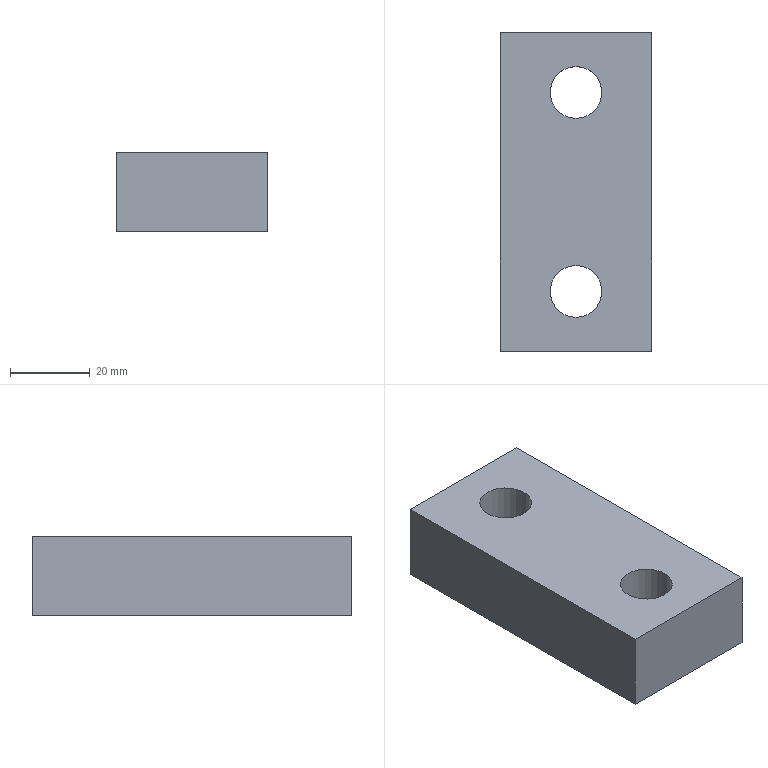Part | NX | features solid 2 | 1 solid | 12 faces | box 38 x 80 x 20 mm | volume 51862 mm3 | plane 8 | cylinder 4 | commonest cylinder face diameters 13 x2 20 x2
STEP:
#1=CARTESIAN_POINT('',(86.,140.,255.));
#2=VERTEX_POINT('',#1);
#3=CARTESIAN_POINT('',(76.,140.,255.));
#4=DIRECTION('',(0.,0.,-1.));
#5=DIRECTION('',(1.,0.,0.));
#6=AXIS2_PLACEMENT_3D('',#3,#4,#5);
#7=CIRCLE('',#6,10.);
#8=EDGE_CURVE('',#2,#2,#7,.F.);
#9=ORIENTED_EDGE('',*,*,#8,.T.);
#10=EDGE_LOOP('',(#9));
#11=FACE_BOUND('',#10,.T.);
#12=CARTESIAN_POINT('',(86.,190.,255.));
#13=VERTEX_POINT('',#12);
#14=CARTESIAN_POINT('',(76.,190.,255.));
#15=DIRECTION('',(0.,0.,-1.));
#16=DIRECTION('',(1.,0.,0.));
#17=AXIS2_PLACEMENT_3D('',#14,#15,#16);
#18=CIRCLE('',#17,10.);
#19=EDGE_CURVE('',#13,#13,#18,.F.);
#20=ORIENTED_EDGE('',*,*,#19,.T.);
#21=EDGE_LOOP('',(#20));
#22=FACE_BOUND('',#21,.T.);
#23=CARTESIAN_POINT('',(95.,125.,255.));
#24=VERTEX_POINT('',#23);
#25=CARTESIAN_POINT('',(95.,205.,255.));
#26=VERTEX_POINT('',#25);
#27=CARTESIAN_POINT('',(95.,165.,255.));
#28=DIRECTION('',(0.,1.,0.));
#29=VECTOR('',#28,1000.);
#30=LINE('',#27,#29);
#31=EDGE_CURVE('',#24,#26,#30,.T.);
#32=ORIENTED_EDGE('',*,*,#31,.F.);
#33=CARTESIAN_POINT('',(57.,125.,255.));
#34=VERTEX_POINT('',#33);
#35=CARTESIAN_POINT('',(75.,125.,255.));
#36=DIRECTION('',(1.,0.,0.));
#37=VECTOR('',#36,1000.);
#38=LINE('',#35,#37);
#39=EDGE_CURVE('',#34,#24,#38,.T.);
#40=ORIENTED_EDGE('',*,*,#39,.F.);
#41=CARTESIAN_POINT('',(57.,205.,255.));
#42=VERTEX_POINT('',#41);
#43=CARTESIAN_POINT('',(57.,165.,255.));
#44=DIRECTION('',(0.,-1.,0.));
#45=VECTOR('',#44,1000.);
#46=LINE('',#43,#45);
#47=EDGE_CURVE('',#42,#34,#46,.T.);
#48=ORIENTED_EDGE('',*,*,#47,.F.);
#49=CARTESIAN_POINT('',(75.,205.,255.));
#50=DIRECTION('',(-1.,0.,0.));
#51=VECTOR('',#50,1000.);
#52=LINE('',#49,#51);
#53=EDGE_CURVE('',#26,#42,#52,.T.);
#54=ORIENTED_EDGE('',*,*,#53,.F.);
#55=EDGE_LOOP('',(#32,#40,#48,#54));
#56=FACE_BOUND('',#55,.T.);
#57=CARTESIAN_POINT('',(75.,165.,255.));
#58=DIRECTION('',(0.,0.,-1.));
#59=DIRECTION('',(0.,-1.,0.));
#60=AXIS2_PLACEMENT_3D('',#57,#58,#59);
#61=PLANE('',#60);
#62=ADVANCED_FACE('',(#11,#22,#56),#61,.T.);
#63=CARTESIAN_POINT('',(95.,125.,275.));
#64=VERTEX_POINT('',#63);
#65=CARTESIAN_POINT('',(95.,125.,260.));
#66=DIRECTION('',(0.,0.,-1.));
#67=VECTOR('',#66,1000.);
#68=LINE('',#65,#67);
#69=EDGE_CURVE('',#64,#24,#68,.T.);
#70=ORIENTED_EDGE('',*,*,#69,.T.);
#71=ORIENTED_EDGE('',*,*,#31,.T.);
#72=CARTESIAN_POINT('',(95.,205.,275.));
#73=VERTEX_POINT('',#72);
#74=CARTESIAN_POINT('',(95.,205.,260.));
#75=DIRECTION('',(0.,0.,-1.));
#76=VECTOR('',#75,1000.);
#77=LINE('',#74,#76);
#78=EDGE_CURVE('',#73,#26,#77,.T.);
#79=ORIENTED_EDGE('',*,*,#78,.F.);
#80=CARTESIAN_POINT('',(95.,165.,275.));
#81=DIRECTION('',(0.,-1.,0.));
#82=VECTOR('',#81,1000.);
#83=LINE('',#80,#82);
#84=EDGE_CURVE('',#73,#64,#83,.T.);
#85=ORIENTED_EDGE('',*,*,#84,.T.);
#86=EDGE_LOOP('',(#70,#71,#79,#85));
#87=FACE_BOUND('',#86,.T.);
#88=CARTESIAN_POINT('',(95.,165.,260.));
#89=DIRECTION('',(1.,0.,0.));
#90=DIRECTION('',(0.,0.,1.));
#91=AXIS2_PLACEMENT_3D('',#88,#89,#90);
#92=PLANE('',#91);
#93=ADVANCED_FACE('',(#87),#92,.T.);
#94=ORIENTED_EDGE('',*,*,#78,.T.);
#95=ORIENTED_EDGE('',*,*,#53,.T.);
#96=CARTESIAN_POINT('',(57.,205.,275.));
#97=VERTEX_POINT('',#96);
#98=CARTESIAN_POINT('',(57.,205.,260.));
#99=DIRECTION('',(0.,0.,-1.));
#100=VECTOR('',#99,1000.);
#101=LINE('',#98,#100);
#102=EDGE_CURVE('',#97,#42,#101,.T.);
#103=ORIENTED_EDGE('',*,*,#102,.F.);
#104=CARTESIAN_POINT('',(75.,205.,275.));
#105=DIRECTION('',(1.,0.,0.));
#106=VECTOR('',#105,1000.);
#107=LINE('',#104,#106);
#108=EDGE_CURVE('',#97,#73,#107,.T.);
#109=ORIENTED_EDGE('',*,*,#108,.T.);
#110=EDGE_LOOP('',(#94,#95,#103,#109));
#111=FACE_BOUND('',#110,.T.);
#112=CARTESIAN_POINT('',(75.,205.,260.));
#113=DIRECTION('',(0.,1.,0.));
#114=DIRECTION('',(0.,0.,-1.));
#115=AXIS2_PLACEMENT_3D('',#112,#113,#114);
#116=PLANE('',#115);
#117=ADVANCED_FACE('',(#111),#116,.T.);
#118=ORIENTED_EDGE('',*,*,#102,.T.);
#119=ORIENTED_EDGE('',*,*,#47,.T.);
#120=CARTESIAN_POINT('',(57.,125.,275.));
#121=VERTEX_POINT('',#120);
#122=CARTESIAN_POINT('',(57.,125.,260.));
#123=DIRECTION('',(0.,0.,-1.));
#124=VECTOR('',#123,1000.);
#125=LINE('',#122,#124);
#126=EDGE_CURVE('',#121,#34,#125,.T.);
#127=ORIENTED_EDGE('',*,*,#126,.F.);
#128=CARTESIAN_POINT('',(57.,165.,275.));
#129=DIRECTION('',(0.,1.,0.));
#130=VECTOR('',#129,1000.);
#131=LINE('',#128,#130);
#132=EDGE_CURVE('',#121,#97,#131,.T.);
#133=ORIENTED_EDGE('',*,*,#132,.T.);
#134=EDGE_LOOP('',(#118,#119,#127,#133));
#135=FACE_BOUND('',#134,.T.);
#136=CARTESIAN_POINT('',(57.,165.,260.));
#137=DIRECTION('',(-1.,0.,0.));
#138=DIRECTION('',(0.,0.,-1.));
#139=AXIS2_PLACEMENT_3D('',#136,#137,#138);
#140=PLANE('',#139);
#141=ADVANCED_FACE('',(#135),#140,.T.);
#142=CARTESIAN_POINT('',(76.,146.5,275.));
#143=VERTEX_POINT('',#142);
#144=CARTESIAN_POINT('',(76.,140.,275.));
#145=DIRECTION('',(0.,0.,1.));
#146=DIRECTION('',(0.,1.,0.));
#147=AXIS2_PLACEMENT_3D('',#144,#145,#146);
#148=CIRCLE('',#147,6.5);
#149=EDGE_CURVE('',#143,#143,#148,.T.);
#150=ORIENTED_EDGE('',*,*,#149,.F.);
#151=EDGE_LOOP('',(#150));
#152=FACE_BOUND('',#151,.T.);
#153=CARTESIAN_POINT('',(76.,196.5,275.));
#154=VERTEX_POINT('',#153);
#155=CARTESIAN_POINT('',(76.,190.,275.));
#156=DIRECTION('',(0.,0.,1.));
#157=DIRECTION('',(0.,1.,0.));
#158=AXIS2_PLACEMENT_3D('',#155,#156,#157);
#159=CIRCLE('',#158,6.5);
#160=EDGE_CURVE('',#154,#154,#159,.T.);
#161=ORIENTED_EDGE('',*,*,#160,.F.);
#162=EDGE_LOOP('',(#161));
#163=FACE_BOUND('',#162,.T.);
#164=CARTESIAN_POINT('',(75.,125.,275.));
#165=DIRECTION('',(-1.,0.,0.));
#166=VECTOR('',#165,1000.);
#167=LINE('',#164,#166);
#168=EDGE_CURVE('',#64,#121,#167,.T.);
#169=ORIENTED_EDGE('',*,*,#168,.F.);
#170=ORIENTED_EDGE('',*,*,#84,.F.);
#171=ORIENTED_EDGE('',*,*,#108,.F.);
#172=ORIENTED_EDGE('',*,*,#132,.F.);
#173=EDGE_LOOP('',(#169,#170,#171,#172));
#174=FACE_BOUND('',#173,.T.);
#175=CARTESIAN_POINT('',(75.,165.,275.));
#176=DIRECTION('',(0.,0.,1.));
#177=DIRECTION('',(0.,1.,0.));
#178=AXIS2_PLACEMENT_3D('',#175,#176,#177);
#179=PLANE('',#178);
#180=ADVANCED_FACE('',(#152,#163,#174),#179,.T.);
#181=ORIENTED_EDGE('',*,*,#168,.T.);
#182=ORIENTED_EDGE('',*,*,#126,.T.);
#183=ORIENTED_EDGE('',*,*,#39,.T.);
#184=ORIENTED_EDGE('',*,*,#69,.F.);
#185=EDGE_LOOP('',(#181,#182,#183,#184));
#186=FACE_BOUND('',#185,.T.);
#187=CARTESIAN_POINT('',(75.,125.,260.));
#188=DIRECTION('',(0.,-1.,0.));
#189=DIRECTION('',(0.,0.,1.));
#190=AXIS2_PLACEMENT_3D('',#187,#188,#189);
#191=PLANE('',#190);
#192=ADVANCED_FACE('',(#186),#191,.T.);
#193=ORIENTED_EDGE('',*,*,#160,.T.);
#194=EDGE_LOOP('',(#193));
#195=FACE_BOUND('',#194,.T.);
#196=CARTESIAN_POINT('',(76.,196.5,265.));
#197=VERTEX_POINT('',#196);
#198=CARTESIAN_POINT('',(76.,190.,265.));
#199=DIRECTION('',(0.,0.,1.));
#200=DIRECTION('',(0.,1.,0.));
#201=AXIS2_PLACEMENT_3D('',#198,#199,#200);
#202=CIRCLE('',#201,6.5);
#203=EDGE_CURVE('',#197,#197,#202,.T.);
#204=ORIENTED_EDGE('',*,*,#203,.F.);
#205=EDGE_LOOP('',(#204));
#206=FACE_BOUND('',#205,.T.);
#207=CARTESIAN_POINT('',(76.,190.,290.));
#208=DIRECTION('',(0.,0.,1.));
#209=DIRECTION('',(0.,1.,0.));
#210=AXIS2_PLACEMENT_3D('',#207,#208,#209);
#211=CYLINDRICAL_SURFACE('',#210,6.5);
#212=ADVANCED_FACE('',(#195,#206),#211,.F.);
#213=ORIENTED_EDGE('',*,*,#203,.T.);
#214=EDGE_LOOP('',(#213));
#215=FACE_BOUND('',#214,.T.);
#216=CARTESIAN_POINT('',(76.,200.,265.));
#217=VERTEX_POINT('',#216);
#218=CARTESIAN_POINT('',(76.,190.,265.));
#219=DIRECTION('',(0.,0.,1.));
#220=DIRECTION('',(0.,1.,0.));
#221=AXIS2_PLACEMENT_3D('',#218,#219,#220);
#222=CIRCLE('',#221,10.);
#223=EDGE_CURVE('',#217,#217,#222,.T.);
#224=ORIENTED_EDGE('',*,*,#223,.F.);
#225=EDGE_LOOP('',(#224));
#226=FACE_BOUND('',#225,.T.);
#227=CARTESIAN_POINT('',(75.,190.,265.));
#228=DIRECTION('',(0.,0.,1.));
#229=DIRECTION('',(0.,1.,0.));
#230=AXIS2_PLACEMENT_3D('',#227,#228,#229);
#231=PLANE('',#230);
#232=ADVANCED_FACE('',(#215,#226),#231,.F.);
#233=ORIENTED_EDGE('',*,*,#223,.T.);
#234=EDGE_LOOP('',(#233));
#235=FACE_BOUND('',#234,.T.);
#236=ORIENTED_EDGE('',*,*,#19,.F.);
#237=EDGE_LOOP('',(#236));
#238=FACE_BOUND('',#237,.T.);
#239=CARTESIAN_POINT('',(76.,190.,240.));
#240=DIRECTION('',(0.,0.,1.));
#241=DIRECTION('',(0.,1.,0.));
#242=AXIS2_PLACEMENT_3D('',#239,#240,#241);
#243=CYLINDRICAL_SURFACE('',#242,10.);
#244=ADVANCED_FACE('',(#235,#238),#243,.F.);
#245=ORIENTED_EDGE('',*,*,#149,.T.);
#246=EDGE_LOOP('',(#245));
#247=FACE_BOUND('',#246,.T.);
#248=CARTESIAN_POINT('',(76.,146.5,265.));
#249=VERTEX_POINT('',#248);
#250=CARTESIAN_POINT('',(76.,140.,265.));
#251=DIRECTION('',(0.,0.,1.));
#252=DIRECTION('',(0.,1.,0.));
#253=AXIS2_PLACEMENT_3D('',#250,#251,#252);
#254=CIRCLE('',#253,6.5);
#255=EDGE_CURVE('',#249,#249,#254,.T.);
#256=ORIENTED_EDGE('',*,*,#255,.F.);
#257=EDGE_LOOP('',(#256));
#258=FACE_BOUND('',#257,.T.);
#259=CARTESIAN_POINT('',(76.,140.,290.));
#260=DIRECTION('',(0.,0.,1.));
#261=DIRECTION('',(0.,1.,0.));
#262=AXIS2_PLACEMENT_3D('',#259,#260,#261);
#263=CYLINDRICAL_SURFACE('',#262,6.5);
#264=ADVANCED_FACE('',(#247,#258),#263,.F.);
#265=ORIENTED_EDGE('',*,*,#255,.T.);
#266=EDGE_LOOP('',(#265));
#267=FACE_BOUND('',#266,.T.);
#268=CARTESIAN_POINT('',(76.,150.,265.));
#269=VERTEX_POINT('',#268);
#270=CARTESIAN_POINT('',(76.,140.,265.));
#271=DIRECTION('',(0.,0.,1.));
#272=DIRECTION('',(0.,1.,0.));
#273=AXIS2_PLACEMENT_3D('',#270,#271,#272);
#274=CIRCLE('',#273,10.);
#275=EDGE_CURVE('',#269,#269,#274,.T.);
#276=ORIENTED_EDGE('',*,*,#275,.F.);
#277=EDGE_LOOP('',(#276));
#278=FACE_BOUND('',#277,.T.);
#279=CARTESIAN_POINT('',(75.,140.,265.));
#280=DIRECTION('',(0.,0.,1.));
#281=DIRECTION('',(0.,1.,0.));
#282=AXIS2_PLACEMENT_3D('',#279,#280,#281);
#283=PLANE('',#282);
#284=ADVANCED_FACE('',(#267,#278),#283,.F.);
#285=ORIENTED_EDGE('',*,*,#275,.T.);
#286=EDGE_LOOP('',(#285));
#287=FACE_BOUND('',#286,.T.);
#288=ORIENTED_EDGE('',*,*,#8,.F.);
#289=EDGE_LOOP('',(#288));
#290=FACE_BOUND('',#289,.T.);
#291=CARTESIAN_POINT('',(76.,140.,240.));
#292=DIRECTION('',(0.,0.,1.));
#293=DIRECTION('',(0.,1.,0.));
#294=AXIS2_PLACEMENT_3D('',#291,#292,#293);
#295=CYLINDRICAL_SURFACE('',#294,10.);
#296=ADVANCED_FACE('',(#287,#290),#295,.F.);
#297=CLOSED_SHELL('',(#62,#93,#117,#141,#180,#192,#212,#232,#244,#264,#284,#296));
#298=MANIFOLD_SOLID_BREP('',#297);
#299=(LENGTH_UNIT()NAMED_UNIT(*)SI_UNIT(.MILLI.,.METRE.));
#300=UNCERTAINTY_MEASURE_WITH_UNIT(LENGTH_MEASURE(0.00001),#299,'','');
#301=(NAMED_UNIT(*)PLANE_ANGLE_UNIT()SI_UNIT($,.RADIAN.));
#302=(NAMED_UNIT(*)SI_UNIT($,.STERADIAN.)SOLID_ANGLE_UNIT());
#303=(GEOMETRIC_REPRESENTATION_CONTEXT(3)GLOBAL_UNCERTAINTY_ASSIGNED_CONTEXT((#300))GLOBAL_UNIT_ASSIGNED_CONTEXT((#299,#301,#302))REPRESENTATION_CONTEXT('',''));
#304=ADVANCED_BREP_SHAPE_REPRESENTATION('',(#298),#303);